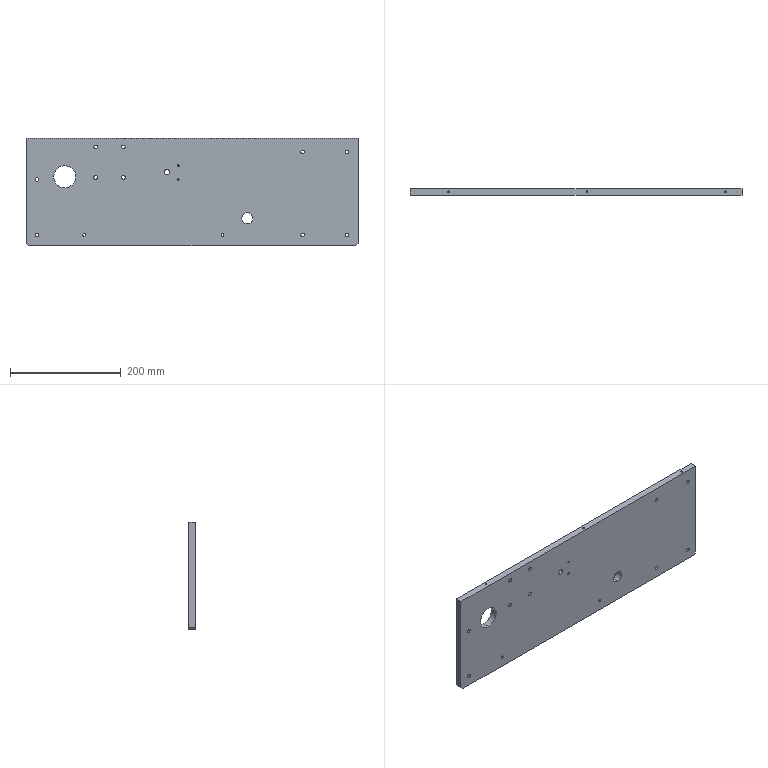Part | SolidWorks | features 3DProfileFeature 5, HoleWzd 5, Cut 3, Chamfer 1, Extrusion 1 | 1 solid | 72 faces | box 600 x 12 x 195 mm | volume 1376203 mm3 | cylinder 52 | plane 14 | cone 6 | commonest cylinder face diameters 6.6 x12 11 x12 3.3 x10 6.8 x8 5 x4 10 x2